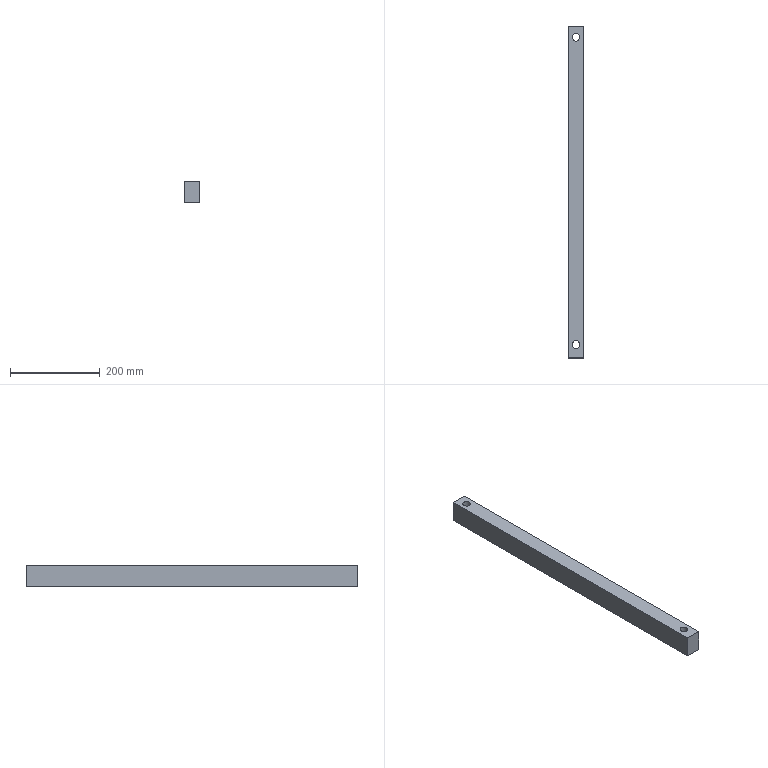Part | NX | features solid 2 | 1 solid | 8 faces | box 35 x 740 x 49 mm | volume 1246856 mm3 | plane 6 | cylinder 2 | commonest cylinder face diameters 17 x2
STEP:
#1=CARTESIAN_POINT('',(20.5,370.,153.));
#2=VERTEX_POINT('',#1);
#3=CARTESIAN_POINT('',(20.5,370.,202.));
#4=VERTEX_POINT('',#3);
#5=CARTESIAN_POINT('',(20.5,370.,148.));
#6=DIRECTION('',(0.,0.,1.));
#7=VECTOR('',#6,1000.);
#8=LINE('',#5,#7);
#9=EDGE_CURVE('',#2,#4,#8,.T.);
#10=ORIENTED_EDGE('',*,*,#9,.F.);
#11=CARTESIAN_POINT('',(20.5,-370.,153.));
#12=VERTEX_POINT('',#11);
#13=CARTESIAN_POINT('',(20.5,0.,153.));
#14=DIRECTION('',(0.,-1.,0.));
#15=VECTOR('',#14,1000.);
#16=LINE('',#13,#15);
#17=EDGE_CURVE('',#2,#12,#16,.T.);
#18=ORIENTED_EDGE('',*,*,#17,.T.);
#19=CARTESIAN_POINT('',(20.5,-370.,202.));
#20=VERTEX_POINT('',#19);
#21=CARTESIAN_POINT('',(20.5,-370.,148.));
#22=DIRECTION('',(0.,0.,1.));
#23=VECTOR('',#22,1000.);
#24=LINE('',#21,#23);
#25=EDGE_CURVE('',#12,#20,#24,.T.);
#26=ORIENTED_EDGE('',*,*,#25,.T.);
#27=CARTESIAN_POINT('',(20.5,0.,202.));
#28=DIRECTION('',(0.,1.,0.));
#29=VECTOR('',#28,1000.);
#30=LINE('',#27,#29);
#31=EDGE_CURVE('',#20,#4,#30,.T.);
#32=ORIENTED_EDGE('',*,*,#31,.T.);
#33=EDGE_LOOP('',(#10,#18,#26,#32));
#34=FACE_BOUND('',#33,.T.);
#35=CARTESIAN_POINT('',(20.5,0.,148.));
#36=DIRECTION('',(-1.,0.,0.));
#37=DIRECTION('',(0.,0.,1.));
#38=AXIS2_PLACEMENT_3D('',#35,#36,#37);
#39=PLANE('',#38);
#40=ADVANCED_FACE('',(#34),#39,.T.);
#41=CARTESIAN_POINT('',(29.5,-340.,202.));
#42=VERTEX_POINT('',#41);
#43=CARTESIAN_POINT('',(38.,-340.,202.));
#44=DIRECTION('',(0.,0.,1.));
#45=DIRECTION('',(-1.,0.,0.));
#46=AXIS2_PLACEMENT_3D('',#43,#44,#45);
#47=CIRCLE('',#46,8.5);
#48=EDGE_CURVE('',#42,#42,#47,.F.);
#49=ORIENTED_EDGE('',*,*,#48,.F.);
#50=EDGE_LOOP('',(#49));
#51=FACE_BOUND('',#50,.T.);
#52=CARTESIAN_POINT('',(29.5,-340.,153.));
#53=VERTEX_POINT('',#52);
#54=CARTESIAN_POINT('',(38.,-340.,153.));
#55=DIRECTION('',(0.,0.,-1.));
#56=DIRECTION('',(-1.,0.,0.));
#57=AXIS2_PLACEMENT_3D('',#54,#55,#56);
#58=CIRCLE('',#57,8.5);
#59=EDGE_CURVE('',#53,#53,#58,.F.);
#60=ORIENTED_EDGE('',*,*,#59,.F.);
#61=EDGE_LOOP('',(#60));
#62=FACE_BOUND('',#61,.T.);
#63=CARTESIAN_POINT('',(38.,-340.,202.));
#64=DIRECTION('',(0.,0.,-1.));
#65=DIRECTION('',(-1.,0.,0.));
#66=AXIS2_PLACEMENT_3D('',#63,#64,#65);
#67=CYLINDRICAL_SURFACE('',#66,8.5);
#68=ADVANCED_FACE('',(#51,#62),#67,.F.);
#69=CARTESIAN_POINT('',(55.5,370.,153.));
#70=VERTEX_POINT('',#69);
#71=CARTESIAN_POINT('',(55.5,370.,202.));
#72=VERTEX_POINT('',#71);
#73=CARTESIAN_POINT('',(55.5,370.,148.));
#74=DIRECTION('',(0.,0.,1.));
#75=VECTOR('',#74,1000.);
#76=LINE('',#73,#75);
#77=EDGE_CURVE('',#70,#72,#76,.T.);
#78=ORIENTED_EDGE('',*,*,#77,.F.);
#79=CARTESIAN_POINT('',(38.,370.,153.));
#80=DIRECTION('',(-1.,0.,0.));
#81=VECTOR('',#80,1000.);
#82=LINE('',#79,#81);
#83=EDGE_CURVE('',#70,#2,#82,.T.);
#84=ORIENTED_EDGE('',*,*,#83,.T.);
#85=ORIENTED_EDGE('',*,*,#9,.T.);
#86=CARTESIAN_POINT('',(38.,370.,202.));
#87=DIRECTION('',(1.,0.,0.));
#88=VECTOR('',#87,1000.);
#89=LINE('',#86,#88);
#90=EDGE_CURVE('',#4,#72,#89,.T.);
#91=ORIENTED_EDGE('',*,*,#90,.T.);
#92=EDGE_LOOP('',(#78,#84,#85,#91));
#93=FACE_BOUND('',#92,.T.);
#94=CARTESIAN_POINT('',(38.,370.,148.));
#95=DIRECTION('',(0.,1.,0.));
#96=DIRECTION('',(0.,0.,1.));
#97=AXIS2_PLACEMENT_3D('',#94,#95,#96);
#98=PLANE('',#97);
#99=ADVANCED_FACE('',(#93),#98,.T.);
#100=CARTESIAN_POINT('',(55.5,-370.,153.));
#101=VERTEX_POINT('',#100);
#102=CARTESIAN_POINT('',(55.5,-370.,202.));
#103=VERTEX_POINT('',#102);
#104=CARTESIAN_POINT('',(55.5,-370.,148.));
#105=DIRECTION('',(0.,0.,1.));
#106=VECTOR('',#105,1000.);
#107=LINE('',#104,#106);
#108=EDGE_CURVE('',#101,#103,#107,.T.);
#109=ORIENTED_EDGE('',*,*,#108,.F.);
#110=CARTESIAN_POINT('',(55.5,0.,153.));
#111=DIRECTION('',(0.,1.,0.));
#112=VECTOR('',#111,1000.);
#113=LINE('',#110,#112);
#114=EDGE_CURVE('',#101,#70,#113,.T.);
#115=ORIENTED_EDGE('',*,*,#114,.T.);
#116=ORIENTED_EDGE('',*,*,#77,.T.);
#117=CARTESIAN_POINT('',(55.5,0.,202.));
#118=DIRECTION('',(0.,-1.,0.));
#119=VECTOR('',#118,1000.);
#120=LINE('',#117,#119);
#121=EDGE_CURVE('',#72,#103,#120,.T.);
#122=ORIENTED_EDGE('',*,*,#121,.T.);
#123=EDGE_LOOP('',(#109,#115,#116,#122));
#124=FACE_BOUND('',#123,.T.);
#125=CARTESIAN_POINT('',(55.5,0.,148.));
#126=DIRECTION('',(1.,0.,0.));
#127=DIRECTION('',(0.,0.,-1.));
#128=AXIS2_PLACEMENT_3D('',#125,#126,#127);
#129=PLANE('',#128);
#130=ADVANCED_FACE('',(#124),#129,.T.);
#131=ORIENTED_EDGE('',*,*,#25,.F.);
#132=CARTESIAN_POINT('',(38.,-370.,153.));
#133=DIRECTION('',(1.,0.,0.));
#134=VECTOR('',#133,1000.);
#135=LINE('',#132,#134);
#136=EDGE_CURVE('',#12,#101,#135,.T.);
#137=ORIENTED_EDGE('',*,*,#136,.T.);
#138=ORIENTED_EDGE('',*,*,#108,.T.);
#139=CARTESIAN_POINT('',(38.,-370.,202.));
#140=DIRECTION('',(-1.,0.,0.));
#141=VECTOR('',#140,1000.);
#142=LINE('',#139,#141);
#143=EDGE_CURVE('',#103,#20,#142,.T.);
#144=ORIENTED_EDGE('',*,*,#143,.T.);
#145=EDGE_LOOP('',(#131,#137,#138,#144));
#146=FACE_BOUND('',#145,.T.);
#147=CARTESIAN_POINT('',(38.,-370.,148.));
#148=DIRECTION('',(0.,-1.,0.));
#149=DIRECTION('',(0.,0.,-1.));
#150=AXIS2_PLACEMENT_3D('',#147,#148,#149);
#151=PLANE('',#150);
#152=ADVANCED_FACE('',(#146),#151,.T.);
#153=CARTESIAN_POINT('',(29.5,345.,202.));
#154=VERTEX_POINT('',#153);
#155=CARTESIAN_POINT('',(38.,345.,202.));
#156=DIRECTION('',(0.,0.,-1.));
#157=DIRECTION('',(-1.,0.,0.));
#158=AXIS2_PLACEMENT_3D('',#155,#156,#157);
#159=CIRCLE('',#158,8.5);
#160=EDGE_CURVE('',#154,#154,#159,.T.);
#161=ORIENTED_EDGE('',*,*,#160,.F.);
#162=EDGE_LOOP('',(#161));
#163=FACE_BOUND('',#162,.T.);
#164=CARTESIAN_POINT('',(29.5,345.,153.));
#165=VERTEX_POINT('',#164);
#166=CARTESIAN_POINT('',(38.,345.,153.));
#167=DIRECTION('',(0.,0.,-1.));
#168=DIRECTION('',(-1.,0.,0.));
#169=AXIS2_PLACEMENT_3D('',#166,#167,#168);
#170=CIRCLE('',#169,8.5);
#171=EDGE_CURVE('',#165,#165,#170,.F.);
#172=ORIENTED_EDGE('',*,*,#171,.F.);
#173=EDGE_LOOP('',(#172));
#174=FACE_BOUND('',#173,.T.);
#175=CARTESIAN_POINT('',(38.,345.,202.));
#176=DIRECTION('',(0.,0.,-1.));
#177=DIRECTION('',(-1.,0.,0.));
#178=AXIS2_PLACEMENT_3D('',#175,#176,#177);
#179=CYLINDRICAL_SURFACE('',#178,8.5);
#180=ADVANCED_FACE('',(#163,#174),#179,.F.);
#181=ORIENTED_EDGE('',*,*,#48,.T.);
#182=EDGE_LOOP('',(#181));
#183=FACE_BOUND('',#182,.T.);
#184=ORIENTED_EDGE('',*,*,#160,.T.);
#185=EDGE_LOOP('',(#184));
#186=FACE_BOUND('',#185,.T.);
#187=ORIENTED_EDGE('',*,*,#90,.F.);
#188=ORIENTED_EDGE('',*,*,#31,.F.);
#189=ORIENTED_EDGE('',*,*,#143,.F.);
#190=ORIENTED_EDGE('',*,*,#121,.F.);
#191=EDGE_LOOP('',(#187,#188,#189,#190));
#192=FACE_BOUND('',#191,.T.);
#193=CARTESIAN_POINT('',(38.,0.,202.));
#194=DIRECTION('',(0.,0.,1.));
#195=DIRECTION('',(1.,0.,0.));
#196=AXIS2_PLACEMENT_3D('',#193,#194,#195);
#197=PLANE('',#196);
#198=ADVANCED_FACE('',(#183,#186,#192),#197,.T.);
#199=ORIENTED_EDGE('',*,*,#171,.T.);
#200=EDGE_LOOP('',(#199));
#201=FACE_BOUND('',#200,.T.);
#202=ORIENTED_EDGE('',*,*,#17,.F.);
#203=ORIENTED_EDGE('',*,*,#83,.F.);
#204=ORIENTED_EDGE('',*,*,#114,.F.);
#205=ORIENTED_EDGE('',*,*,#136,.F.);
#206=EDGE_LOOP('',(#202,#203,#204,#205));
#207=FACE_BOUND('',#206,.T.);
#208=ORIENTED_EDGE('',*,*,#59,.T.);
#209=EDGE_LOOP('',(#208));
#210=FACE_BOUND('',#209,.T.);
#211=CARTESIAN_POINT('',(765.,0.,153.));
#212=DIRECTION('',(0.,0.,-1.));
#213=DIRECTION('',(-1.,0.,0.));
#214=AXIS2_PLACEMENT_3D('',#211,#212,#213);
#215=PLANE('',#214);
#216=ADVANCED_FACE('',(#201,#207,#210),#215,.T.);
#217=CLOSED_SHELL('',(#40,#68,#99,#130,#152,#180,#198,#216));
#218=MANIFOLD_SOLID_BREP('',#217);
#219=(LENGTH_UNIT()NAMED_UNIT(*)SI_UNIT(.MILLI.,.METRE.));
#220=UNCERTAINTY_MEASURE_WITH_UNIT(LENGTH_MEASURE(0.00001),#219,'','');
#221=(NAMED_UNIT(*)PLANE_ANGLE_UNIT()SI_UNIT($,.RADIAN.));
#222=(NAMED_UNIT(*)SI_UNIT($,.STERADIAN.)SOLID_ANGLE_UNIT());
#223=(GEOMETRIC_REPRESENTATION_CONTEXT(3)GLOBAL_UNCERTAINTY_ASSIGNED_CONTEXT((#220))GLOBAL_UNIT_ASSIGNED_CONTEXT((#219,#221,#222))REPRESENTATION_CONTEXT('',''));
#224=ADVANCED_BREP_SHAPE_REPRESENTATION('',(#218),#223);